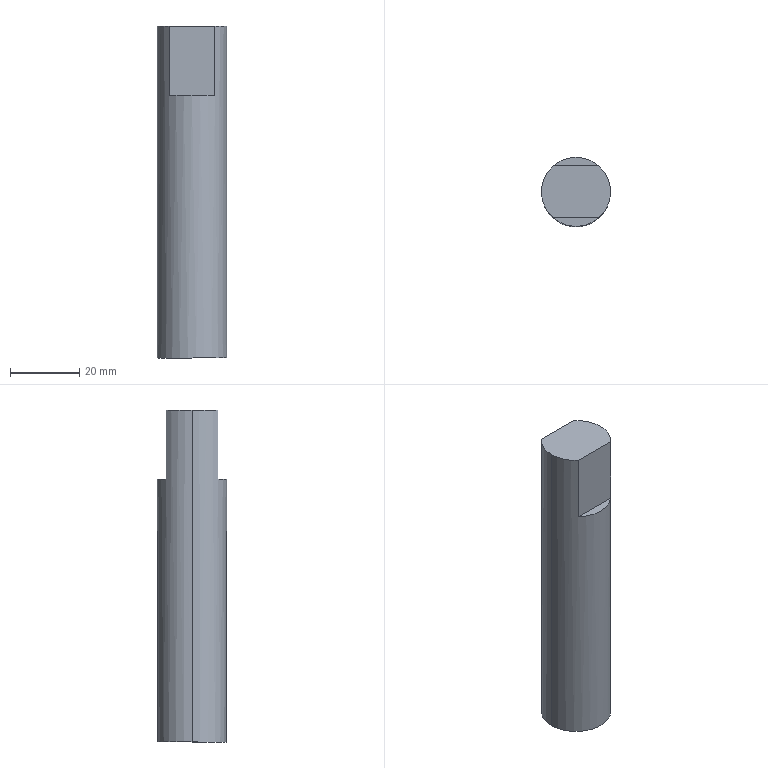Part | STEP file | 1 solid | 8 faces | box 20 x 20 x 96 mm | volume 29253 mm3 | plane 6 | cylinder 2 | commonest cylinder face diameters 20 x2
STEP:
#1=CARTESIAN_POINT('',(0.,0.,0.));
#2=DIRECTION('',(0.,0.,1.));
#3=DIRECTION('',(1.,0.,0.));
#4=AXIS2_PLACEMENT_3D('',#1,#2,#3);
#5=CARTESIAN_POINT('',(-51.732,1772.5,60.));
#6=VERTEX_POINT('',#5);
#7=CARTESIAN_POINT('',(-38.503,1772.5,60.));
#8=VERTEX_POINT('',#7);
#9=CARTESIAN_POINT('',(-45.117,1772.5,60.));
#10=DIRECTION('',(1.,0.,0.));
#11=VECTOR('',#10,1.);
#12=LINE('',#9,#11);
#13=CARTESIAN_POINT('',(-57.617,1772.5,40.));
#14=DIRECTION('',(0.,-1.,0.));
#15=DIRECTION('',(0.,0.,-1.));
#16=AXIS2_PLACEMENT_3D('',#13,#14,#15);
#17=PLANE('',#16);
#18=CARTESIAN_POINT('',(-20.,12.5));
#19=DIRECTION('',(0.,1.));
#20=VECTOR('',#19,1.);
#21=LINE('',#18,#20);
#22=(GEOMETRIC_REPRESENTATION_CONTEXT(2)PARAMETRIC_REPRESENTATION_CONTEXT()REPRESENTATION_CONTEXT('',''));
#23=DEFINITIONAL_REPRESENTATION('',(#21),#22);
#24=PCURVE('',#17,#23);
#25=CARTESIAN_POINT('',(-45.117,1780.,60.));
#26=DIRECTION('',(0.,0.,1.));
#27=DIRECTION('',(0.,-1.,0.));
#28=AXIS2_PLACEMENT_3D('',#25,#26,#27);
#29=PLANE('',#28);
#30=CARTESIAN_POINT('',(7.5,0.));
#31=DIRECTION('',(0.,1.));
#32=VECTOR('',#31,1.);
#33=LINE('',#30,#32);
#34=(GEOMETRIC_REPRESENTATION_CONTEXT(2)PARAMETRIC_REPRESENTATION_CONTEXT()REPRESENTATION_CONTEXT('',''));
#35=DEFINITIONAL_REPRESENTATION('',(#33),#34);
#36=PCURVE('',#29,#35);
#37=SURFACE_CURVE('',#12,(#24,#36),.PCURVE_S1.);
#38=EDGE_CURVE('',#6,#8,#37,.T.);
#39=ORIENTED_EDGE('',*,*,#38,.F.);
#40=CARTESIAN_POINT('',(-51.732,1772.5,40.));
#41=VERTEX_POINT('',#40);
#42=CARTESIAN_POINT('',(-51.732,1772.5,-36.));
#43=DIRECTION('',(0.,0.,1.));
#44=VECTOR('',#43,1.);
#45=LINE('',#42,#44);
#46=CARTESIAN_POINT('',(76.,5.886));
#47=DIRECTION('',(-1.,0.));
#48=VECTOR('',#47,1.);
#49=LINE('',#46,#48);
#50=(GEOMETRIC_REPRESENTATION_CONTEXT(2)PARAMETRIC_REPRESENTATION_CONTEXT()REPRESENTATION_CONTEXT('',''));
#51=DEFINITIONAL_REPRESENTATION('',(#49),#50);
#52=PCURVE('',#17,#51);
#53=CARTESIAN_POINT('',(-45.117,1780.,-36.));
#54=DIRECTION('',(0.,0.,1.));
#55=DIRECTION('',(1.,0.,0.));
#56=AXIS2_PLACEMENT_3D('',#53,#54,#55);
#57=CYLINDRICAL_SURFACE('',#56,10.);
#58=CARTESIAN_POINT('',(3.99,0.));
#59=DIRECTION('',(0.,1.));
#60=VECTOR('',#59,1.);
#61=LINE('',#58,#60);
#62=(GEOMETRIC_REPRESENTATION_CONTEXT(2)PARAMETRIC_REPRESENTATION_CONTEXT()REPRESENTATION_CONTEXT('',''));
#63=DEFINITIONAL_REPRESENTATION('',(#61),#62);
#64=PCURVE('',#57,#63);
#65=SURFACE_CURVE('',#45,(#52,#64),.PCURVE_S1.);
#66=EDGE_CURVE('',#41,#6,#65,.T.);
#67=ORIENTED_EDGE('',*,*,#66,.F.);
#68=CARTESIAN_POINT('',(-38.503,1772.5,40.));
#69=VERTEX_POINT('',#68);
#70=CARTESIAN_POINT('',(-57.617,1772.5,40.));
#71=DIRECTION('',(1.,0.,0.));
#72=VECTOR('',#71,1.);
#73=LINE('',#70,#72);
#74=CARTESIAN_POINT('',(0.,0.));
#75=DIRECTION('',(0.,1.));
#76=VECTOR('',#75,1.);
#77=LINE('',#74,#76);
#78=(GEOMETRIC_REPRESENTATION_CONTEXT(2)PARAMETRIC_REPRESENTATION_CONTEXT()REPRESENTATION_CONTEXT('',''));
#79=DEFINITIONAL_REPRESENTATION('',(#77),#78);
#80=PCURVE('',#17,#79);
#81=CARTESIAN_POINT('',(-45.117,1780.,40.));
#82=DIRECTION('',(0.,0.,1.));
#83=DIRECTION('',(1.,0.,0.));
#84=AXIS2_PLACEMENT_3D('',#81,#82,#83);
#85=PLANE('',#84);
#86=CARTESIAN_POINT('',(-12.5,-7.5));
#87=DIRECTION('',(1.,0.));
#88=VECTOR('',#87,1.);
#89=LINE('',#86,#88);
#90=(GEOMETRIC_REPRESENTATION_CONTEXT(2)PARAMETRIC_REPRESENTATION_CONTEXT()REPRESENTATION_CONTEXT('',''));
#91=DEFINITIONAL_REPRESENTATION('',(#89),#90);
#92=PCURVE('',#85,#91);
#93=SURFACE_CURVE('',#73,(#80,#92),.PCURVE_S1.);
#94=EDGE_CURVE('',#41,#69,#93,.T.);
#95=ORIENTED_EDGE('',*,*,#94,.T.);
#96=CARTESIAN_POINT('',(-38.503,1772.5,-36.));
#97=DIRECTION('',(0.,0.,-1.));
#98=VECTOR('',#97,1.);
#99=LINE('',#96,#98);
#100=CARTESIAN_POINT('',(76.,19.114));
#101=DIRECTION('',(1.,0.));
#102=VECTOR('',#101,1.);
#103=LINE('',#100,#102);
#104=(GEOMETRIC_REPRESENTATION_CONTEXT(2)PARAMETRIC_REPRESENTATION_CONTEXT()REPRESENTATION_CONTEXT('',''));
#105=DEFINITIONAL_REPRESENTATION('',(#103),#104);
#106=PCURVE('',#17,#105);
#107=CARTESIAN_POINT('',(5.435,0.));
#108=DIRECTION('',(0.,-1.));
#109=VECTOR('',#108,1.);
#110=LINE('',#107,#109);
#111=(GEOMETRIC_REPRESENTATION_CONTEXT(2)PARAMETRIC_REPRESENTATION_CONTEXT()REPRESENTATION_CONTEXT('',''));
#112=DEFINITIONAL_REPRESENTATION('',(#110),#111);
#113=PCURVE('',#57,#112);
#114=SURFACE_CURVE('',#99,(#106,#113),.PCURVE_S1.);
#115=EDGE_CURVE('',#8,#69,#114,.T.);
#116=ORIENTED_EDGE('',*,*,#115,.F.);
#117=EDGE_LOOP('',(#39,#67,#95,#116));
#118=FACE_BOUND('',#117,.T.);
#119=ADVANCED_FACE('',(#118),#17,.T.);
#120=ORIENTED_EDGE('',*,*,#94,.F.);
#121=CARTESIAN_POINT('',(-45.117,1780.,40.));
#122=DIRECTION('',(0.,0.,-1.));
#123=DIRECTION('',(1.,0.,0.));
#124=AXIS2_PLACEMENT_3D('',#121,#122,#123);
#125=CIRCLE('',#124,10.);
#126=CARTESIAN_POINT('',(10.,0.));
#127=CARTESIAN_POINT('',(10.,-17.321));
#128=CARTESIAN_POINT('',(-5.,-8.66));
#129=CARTESIAN_POINT('',(-20.,0.));
#130=CARTESIAN_POINT('',(-5.,8.66));
#131=CARTESIAN_POINT('',(10.,17.321));
#132=CARTESIAN_POINT('',(10.,0.));
#133=(BOUNDED_CURVE()B_SPLINE_CURVE(2,(#126,#127,#128,#129,#130,#131,#132),.UNSPECIFIED.,.T.,.F.)B_SPLINE_CURVE_WITH_KNOTS((1,2,2,2,2,1),(-2.094,0.,2.094,4.189,6.283,8.378),.UNSPECIFIED.)CURVE()GEOMETRIC_REPRESENTATION_ITEM()RATIONAL_B_SPLINE_CURVE((1.,0.5,1.,0.5,1.,0.5,1.))REPRESENTATION_ITEM(''));
#134=(GEOMETRIC_REPRESENTATION_CONTEXT(2)PARAMETRIC_REPRESENTATION_CONTEXT()REPRESENTATION_CONTEXT('',''));
#135=DEFINITIONAL_REPRESENTATION('',(#133),#134);
#136=PCURVE('',#85,#135);
#137=CARTESIAN_POINT('',(6.283,76.));
#138=DIRECTION('',(-1.,0.));
#139=VECTOR('',#138,1.);
#140=LINE('',#137,#139);
#141=(GEOMETRIC_REPRESENTATION_CONTEXT(2)PARAMETRIC_REPRESENTATION_CONTEXT()REPRESENTATION_CONTEXT('',''));
#142=DEFINITIONAL_REPRESENTATION('',(#140),#141);
#143=PCURVE('',#57,#142);
#144=SURFACE_CURVE('',#125,(#136,#143),.PCURVE_S1.);
#145=EDGE_CURVE('',#69,#41,#144,.T.);
#146=ORIENTED_EDGE('',*,*,#145,.F.);
#147=EDGE_LOOP('',(#120,#146));
#148=FACE_BOUND('',#147,.T.);
#149=ADVANCED_FACE('',(#148),#85,.T.);
#150=CARTESIAN_POINT('',(-38.503,1787.5,40.));
#151=VERTEX_POINT('',#150);
#152=CARTESIAN_POINT('',(-51.732,1787.5,40.));
#153=VERTEX_POINT('',#152);
#154=CARTESIAN_POINT('',(-57.617,1787.5,40.));
#155=DIRECTION('',(-1.,0.,0.));
#156=VECTOR('',#155,1.);
#157=LINE('',#154,#156);
#158=CARTESIAN_POINT('',(-45.117,1780.,40.));
#159=DIRECTION('',(0.,0.,1.));
#160=DIRECTION('',(1.,0.,0.));
#161=AXIS2_PLACEMENT_3D('',#158,#159,#160);
#162=PLANE('',#161);
#163=CARTESIAN_POINT('',(-12.5,7.5));
#164=DIRECTION('',(-1.,0.));
#165=VECTOR('',#164,1.);
#166=LINE('',#163,#165);
#167=(GEOMETRIC_REPRESENTATION_CONTEXT(2)PARAMETRIC_REPRESENTATION_CONTEXT()REPRESENTATION_CONTEXT('',''));
#168=DEFINITIONAL_REPRESENTATION('',(#166),#167);
#169=PCURVE('',#162,#168);
#170=CARTESIAN_POINT('',(-57.617,1787.5,40.));
#171=DIRECTION('',(0.,1.,0.));
#172=DIRECTION('',(1.,0.,0.));
#173=AXIS2_PLACEMENT_3D('',#170,#171,#172);
#174=PLANE('',#173);
#175=CARTESIAN_POINT('',(0.,0.));
#176=DIRECTION('',(-1.,0.));
#177=VECTOR('',#176,1.);
#178=LINE('',#175,#177);
#179=(GEOMETRIC_REPRESENTATION_CONTEXT(2)PARAMETRIC_REPRESENTATION_CONTEXT()REPRESENTATION_CONTEXT('',''));
#180=DEFINITIONAL_REPRESENTATION('',(#178),#179);
#181=PCURVE('',#174,#180);
#182=SURFACE_CURVE('',#157,(#169,#181),.PCURVE_S1.);
#183=EDGE_CURVE('',#151,#153,#182,.T.);
#184=ORIENTED_EDGE('',*,*,#183,.F.);
#185=CARTESIAN_POINT('',(-45.117,1780.,40.));
#186=DIRECTION('',(0.,0.,-1.));
#187=DIRECTION('',(1.,0.,0.));
#188=AXIS2_PLACEMENT_3D('',#185,#186,#187);
#189=CIRCLE('',#188,10.);
#190=CARTESIAN_POINT('',(10.,0.));
#191=CARTESIAN_POINT('',(10.,-17.321));
#192=CARTESIAN_POINT('',(-5.,-8.66));
#193=CARTESIAN_POINT('',(-20.,0.));
#194=CARTESIAN_POINT('',(-5.,8.66));
#195=CARTESIAN_POINT('',(10.,17.321));
#196=CARTESIAN_POINT('',(10.,0.));
#197=(BOUNDED_CURVE()B_SPLINE_CURVE(2,(#190,#191,#192,#193,#194,#195,#196),.UNSPECIFIED.,.T.,.F.)B_SPLINE_CURVE_WITH_KNOTS((1,2,2,2,2,1),(-2.094,0.,2.094,4.189,6.283,8.378),.UNSPECIFIED.)CURVE()GEOMETRIC_REPRESENTATION_ITEM()RATIONAL_B_SPLINE_CURVE((1.,0.5,1.,0.5,1.,0.5,1.))REPRESENTATION_ITEM(''));
#198=(GEOMETRIC_REPRESENTATION_CONTEXT(2)PARAMETRIC_REPRESENTATION_CONTEXT()REPRESENTATION_CONTEXT('',''));
#199=DEFINITIONAL_REPRESENTATION('',(#197),#198);
#200=PCURVE('',#162,#199);
#201=CARTESIAN_POINT('',(-45.117,1780.,-36.));
#202=DIRECTION('',(0.,0.,1.));
#203=DIRECTION('',(1.,0.,0.));
#204=AXIS2_PLACEMENT_3D('',#201,#202,#203);
#205=CYLINDRICAL_SURFACE('',#204,10.);
#206=CARTESIAN_POINT('',(6.283,76.));
#207=DIRECTION('',(-1.,0.));
#208=VECTOR('',#207,1.);
#209=LINE('',#206,#208);
#210=(GEOMETRIC_REPRESENTATION_CONTEXT(2)PARAMETRIC_REPRESENTATION_CONTEXT()REPRESENTATION_CONTEXT('',''));
#211=DEFINITIONAL_REPRESENTATION('',(#209),#210);
#212=PCURVE('',#205,#211);
#213=SURFACE_CURVE('',#189,(#200,#212),.PCURVE_S1.);
#214=EDGE_CURVE('',#153,#151,#213,.T.);
#215=ORIENTED_EDGE('',*,*,#214,.F.);
#216=EDGE_LOOP('',(#184,#215));
#217=FACE_BOUND('',#216,.T.);
#218=ADVANCED_FACE('',(#217),#162,.T.);
#219=CARTESIAN_POINT('',(-38.503,1787.5,60.));
#220=VERTEX_POINT('',#219);
#221=CARTESIAN_POINT('',(-51.732,1787.5,60.));
#222=VERTEX_POINT('',#221);
#223=CARTESIAN_POINT('',(-45.117,1787.5,60.));
#224=DIRECTION('',(-1.,0.,0.));
#225=VECTOR('',#224,1.);
#226=LINE('',#223,#225);
#227=CARTESIAN_POINT('',(12.5,-20.));
#228=DIRECTION('',(-1.,0.));
#229=VECTOR('',#228,1.);
#230=LINE('',#227,#229);
#231=(GEOMETRIC_REPRESENTATION_CONTEXT(2)PARAMETRIC_REPRESENTATION_CONTEXT()REPRESENTATION_CONTEXT('',''));
#232=DEFINITIONAL_REPRESENTATION('',(#230),#231);
#233=PCURVE('',#174,#232);
#234=CARTESIAN_POINT('',(-7.5,0.));
#235=DIRECTION('',(0.,-1.));
#236=VECTOR('',#235,1.);
#237=LINE('',#234,#236);
#238=(GEOMETRIC_REPRESENTATION_CONTEXT(2)PARAMETRIC_REPRESENTATION_CONTEXT()REPRESENTATION_CONTEXT('',''));
#239=DEFINITIONAL_REPRESENTATION('',(#237),#238);
#240=PCURVE('',#29,#239);
#241=SURFACE_CURVE('',#226,(#233,#240),.PCURVE_S1.);
#242=EDGE_CURVE('',#220,#222,#241,.T.);
#243=ORIENTED_EDGE('',*,*,#242,.F.);
#244=CARTESIAN_POINT('',(-38.503,1787.5,-36.));
#245=DIRECTION('',(0.,0.,1.));
#246=VECTOR('',#245,1.);
#247=LINE('',#244,#246);
#248=CARTESIAN_POINT('',(19.114,76.));
#249=DIRECTION('',(0.,-1.));
#250=VECTOR('',#249,1.);
#251=LINE('',#248,#250);
#252=(GEOMETRIC_REPRESENTATION_CONTEXT(2)PARAMETRIC_REPRESENTATION_CONTEXT()REPRESENTATION_CONTEXT('',''));
#253=DEFINITIONAL_REPRESENTATION('',(#251),#252);
#254=PCURVE('',#174,#253);
#255=CARTESIAN_POINT('',(0.8481,0.));
#256=DIRECTION('',(0.,1.));
#257=VECTOR('',#256,1.);
#258=LINE('',#255,#257);
#259=(GEOMETRIC_REPRESENTATION_CONTEXT(2)PARAMETRIC_REPRESENTATION_CONTEXT()REPRESENTATION_CONTEXT('',''));
#260=DEFINITIONAL_REPRESENTATION('',(#258),#259);
#261=PCURVE('',#205,#260);
#262=SURFACE_CURVE('',#247,(#254,#261),.PCURVE_S1.);
#263=EDGE_CURVE('',#151,#220,#262,.T.);
#264=ORIENTED_EDGE('',*,*,#263,.F.);
#265=ORIENTED_EDGE('',*,*,#183,.T.);
#266=CARTESIAN_POINT('',(-51.732,1787.5,-36.));
#267=DIRECTION('',(0.,0.,-1.));
#268=VECTOR('',#267,1.);
#269=LINE('',#266,#268);
#270=CARTESIAN_POINT('',(5.886,76.));
#271=DIRECTION('',(0.,1.));
#272=VECTOR('',#271,1.);
#273=LINE('',#270,#272);
#274=(GEOMETRIC_REPRESENTATION_CONTEXT(2)PARAMETRIC_REPRESENTATION_CONTEXT()REPRESENTATION_CONTEXT('',''));
#275=DEFINITIONAL_REPRESENTATION('',(#273),#274);
#276=PCURVE('',#174,#275);
#277=CARTESIAN_POINT('',(2.294,0.));
#278=DIRECTION('',(0.,-1.));
#279=VECTOR('',#278,1.);
#280=LINE('',#277,#279);
#281=(GEOMETRIC_REPRESENTATION_CONTEXT(2)PARAMETRIC_REPRESENTATION_CONTEXT()REPRESENTATION_CONTEXT('',''));
#282=DEFINITIONAL_REPRESENTATION('',(#280),#281);
#283=PCURVE('',#205,#282);
#284=SURFACE_CURVE('',#269,(#276,#283),.PCURVE_S1.);
#285=EDGE_CURVE('',#222,#153,#284,.T.);
#286=ORIENTED_EDGE('',*,*,#285,.F.);
#287=EDGE_LOOP('',(#243,#264,#265,#286));
#288=FACE_BOUND('',#287,.T.);
#289=ADVANCED_FACE('',(#288),#174,.T.);
#290=CARTESIAN_POINT('',(-35.117,1780.,-36.));
#291=VERTEX_POINT('',#290);
#292=CARTESIAN_POINT('',(-55.117,1780.,-36.));
#293=VERTEX_POINT('',#292);
#294=CARTESIAN_POINT('',(-45.117,1780.,-36.));
#295=DIRECTION('',(0.,0.,1.));
#296=DIRECTION('',(1.,0.,0.));
#297=AXIS2_PLACEMENT_3D('',#294,#295,#296);
#298=CIRCLE('',#297,10.);
#299=CARTESIAN_POINT('',(-45.117,1780.,-36.));
#300=DIRECTION('',(0.,0.,1.));
#301=DIRECTION('',(0.,-1.,0.));
#302=AXIS2_PLACEMENT_3D('',#299,#300,#301);
#303=PLANE('',#302);
#304=CARTESIAN_POINT('',(0.,0.));
#305=DIRECTION('',(0.,1.));
#306=AXIS2_PLACEMENT_2D('',#304,#305);
#307=CIRCLE('',#306,10.);
#308=(GEOMETRIC_REPRESENTATION_CONTEXT(2)PARAMETRIC_REPRESENTATION_CONTEXT()REPRESENTATION_CONTEXT('',''));
#309=DEFINITIONAL_REPRESENTATION('',(#307),#308);
#310=PCURVE('',#303,#309);
#311=CARTESIAN_POINT('',(0.,0.));
#312=DIRECTION('',(1.,0.));
#313=VECTOR('',#312,1.);
#314=LINE('',#311,#313);
#315=(GEOMETRIC_REPRESENTATION_CONTEXT(2)PARAMETRIC_REPRESENTATION_CONTEXT()REPRESENTATION_CONTEXT('',''));
#316=DEFINITIONAL_REPRESENTATION('',(#314),#315);
#317=PCURVE('',#205,#316);
#318=SURFACE_CURVE('',#298,(#310,#317),.PCURVE_S1.);
#319=EDGE_CURVE('',#291,#293,#318,.T.);
#320=ORIENTED_EDGE('',*,*,#319,.F.);
#321=CARTESIAN_POINT('',(-45.117,1780.,-36.));
#322=DIRECTION('',(0.,0.,1.));
#323=DIRECTION('',(1.,0.,0.));
#324=AXIS2_PLACEMENT_3D('',#321,#322,#323);
#325=CIRCLE('',#324,10.);
#326=CARTESIAN_POINT('',(0.,0.));
#327=DIRECTION('',(0.,1.));
#328=AXIS2_PLACEMENT_2D('',#326,#327);
#329=CIRCLE('',#328,10.);
#330=(GEOMETRIC_REPRESENTATION_CONTEXT(2)PARAMETRIC_REPRESENTATION_CONTEXT()REPRESENTATION_CONTEXT('',''));
#331=DEFINITIONAL_REPRESENTATION('',(#329),#330);
#332=PCURVE('',#303,#331);
#333=CARTESIAN_POINT('',(0.,0.));
#334=DIRECTION('',(1.,0.));
#335=VECTOR('',#334,1.);
#336=LINE('',#333,#335);
#337=(GEOMETRIC_REPRESENTATION_CONTEXT(2)PARAMETRIC_REPRESENTATION_CONTEXT()REPRESENTATION_CONTEXT('',''));
#338=DEFINITIONAL_REPRESENTATION('',(#336),#337);
#339=PCURVE('',#57,#338);
#340=SURFACE_CURVE('',#325,(#332,#339),.PCURVE_S1.);
#341=EDGE_CURVE('',#293,#291,#340,.T.);
#342=ORIENTED_EDGE('',*,*,#341,.F.);
#343=EDGE_LOOP('',(#320,#342));
#344=FACE_BOUND('',#343,.T.);
#345=ADVANCED_FACE('',(#344),#303,.F.);
#346=CARTESIAN_POINT('',(-55.117,1780.,60.));
#347=VERTEX_POINT('',#346);
#348=CARTESIAN_POINT('',(-45.117,1780.,60.));
#349=DIRECTION('',(0.,0.,1.));
#350=DIRECTION('',(1.,0.,0.));
#351=AXIS2_PLACEMENT_3D('',#348,#349,#350);
#352=CIRCLE('',#351,10.);
#353=CARTESIAN_POINT('',(0.,0.));
#354=DIRECTION('',(0.,1.));
#355=AXIS2_PLACEMENT_2D('',#353,#354);
#356=CIRCLE('',#355,10.);
#357=(GEOMETRIC_REPRESENTATION_CONTEXT(2)PARAMETRIC_REPRESENTATION_CONTEXT()REPRESENTATION_CONTEXT('',''));
#358=DEFINITIONAL_REPRESENTATION('',(#356),#357);
#359=PCURVE('',#29,#358);
#360=CARTESIAN_POINT('',(0.,96.));
#361=DIRECTION('',(1.,0.));
#362=VECTOR('',#361,1.);
#363=LINE('',#360,#362);
#364=(GEOMETRIC_REPRESENTATION_CONTEXT(2)PARAMETRIC_REPRESENTATION_CONTEXT()REPRESENTATION_CONTEXT('',''));
#365=DEFINITIONAL_REPRESENTATION('',(#363),#364);
#366=PCURVE('',#205,#365);
#367=SURFACE_CURVE('',#352,(#359,#366),.PCURVE_S1.);
#368=EDGE_CURVE('',#222,#347,#367,.T.);
#369=ORIENTED_EDGE('',*,*,#368,.T.);
#370=CARTESIAN_POINT('',(-45.117,1780.,60.));
#371=DIRECTION('',(0.,0.,1.));
#372=DIRECTION('',(1.,0.,0.));
#373=AXIS2_PLACEMENT_3D('',#370,#371,#372);
#374=CIRCLE('',#373,10.);
#375=CARTESIAN_POINT('',(0.,0.));
#376=DIRECTION('',(0.,1.));
#377=AXIS2_PLACEMENT_2D('',#375,#376);
#378=CIRCLE('',#377,10.);
#379=(GEOMETRIC_REPRESENTATION_CONTEXT(2)PARAMETRIC_REPRESENTATION_CONTEXT()REPRESENTATION_CONTEXT('',''));
#380=DEFINITIONAL_REPRESENTATION('',(#378),#379);
#381=PCURVE('',#29,#380);
#382=CARTESIAN_POINT('',(0.,96.));
#383=DIRECTION('',(1.,0.));
#384=VECTOR('',#383,1.);
#385=LINE('',#382,#384);
#386=(GEOMETRIC_REPRESENTATION_CONTEXT(2)PARAMETRIC_REPRESENTATION_CONTEXT()REPRESENTATION_CONTEXT('',''));
#387=DEFINITIONAL_REPRESENTATION('',(#385),#386);
#388=PCURVE('',#57,#387);
#389=SURFACE_CURVE('',#374,(#381,#388),.PCURVE_S1.);
#390=EDGE_CURVE('',#347,#6,#389,.T.);
#391=ORIENTED_EDGE('',*,*,#390,.T.);
#392=ORIENTED_EDGE('',*,*,#38,.T.);
#393=CARTESIAN_POINT('',(-35.117,1780.,60.));
#394=VERTEX_POINT('',#393);
#395=CARTESIAN_POINT('',(-45.117,1780.,60.));
#396=DIRECTION('',(0.,0.,1.));
#397=DIRECTION('',(1.,0.,0.));
#398=AXIS2_PLACEMENT_3D('',#395,#396,#397);
#399=CIRCLE('',#398,10.);
#400=CARTESIAN_POINT('',(0.,0.));
#401=DIRECTION('',(0.,1.));
#402=AXIS2_PLACEMENT_2D('',#400,#401);
#403=CIRCLE('',#402,10.);
#404=(GEOMETRIC_REPRESENTATION_CONTEXT(2)PARAMETRIC_REPRESENTATION_CONTEXT()REPRESENTATION_CONTEXT('',''));
#405=DEFINITIONAL_REPRESENTATION('',(#403),#404);
#406=PCURVE('',#29,#405);
#407=CARTESIAN_POINT('',(0.,96.));
#408=DIRECTION('',(1.,0.));
#409=VECTOR('',#408,1.);
#410=LINE('',#407,#409);
#411=(GEOMETRIC_REPRESENTATION_CONTEXT(2)PARAMETRIC_REPRESENTATION_CONTEXT()REPRESENTATION_CONTEXT('',''));
#412=DEFINITIONAL_REPRESENTATION('',(#410),#411);
#413=PCURVE('',#57,#412);
#414=SURFACE_CURVE('',#399,(#406,#413),.PCURVE_S1.);
#415=EDGE_CURVE('',#8,#394,#414,.T.);
#416=ORIENTED_EDGE('',*,*,#415,.T.);
#417=CARTESIAN_POINT('',(-45.117,1780.,60.));
#418=DIRECTION('',(0.,0.,1.));
#419=DIRECTION('',(1.,0.,0.));
#420=AXIS2_PLACEMENT_3D('',#417,#418,#419);
#421=CIRCLE('',#420,10.);
#422=CARTESIAN_POINT('',(0.,0.));
#423=DIRECTION('',(0.,1.));
#424=AXIS2_PLACEMENT_2D('',#422,#423);
#425=CIRCLE('',#424,10.);
#426=(GEOMETRIC_REPRESENTATION_CONTEXT(2)PARAMETRIC_REPRESENTATION_CONTEXT()REPRESENTATION_CONTEXT('',''));
#427=DEFINITIONAL_REPRESENTATION('',(#425),#426);
#428=PCURVE('',#29,#427);
#429=CARTESIAN_POINT('',(0.,96.));
#430=DIRECTION('',(1.,0.));
#431=VECTOR('',#430,1.);
#432=LINE('',#429,#431);
#433=(GEOMETRIC_REPRESENTATION_CONTEXT(2)PARAMETRIC_REPRESENTATION_CONTEXT()REPRESENTATION_CONTEXT('',''));
#434=DEFINITIONAL_REPRESENTATION('',(#432),#433);
#435=PCURVE('',#205,#434);
#436=SURFACE_CURVE('',#421,(#428,#435),.PCURVE_S1.);
#437=EDGE_CURVE('',#394,#220,#436,.T.);
#438=ORIENTED_EDGE('',*,*,#437,.T.);
#439=ORIENTED_EDGE('',*,*,#242,.T.);
#440=EDGE_LOOP('',(#369,#391,#392,#416,#438,#439));
#441=FACE_BOUND('',#440,.T.);
#442=ADVANCED_FACE('',(#441),#29,.T.);
#443=CARTESIAN_POINT('',(-55.117,1780.,-36.));
#444=DIRECTION('',(0.,0.,1.));
#445=VECTOR('',#444,1.);
#446=LINE('',#443,#445);
#447=CARTESIAN_POINT('',(3.142,0.));
#448=DIRECTION('',(0.,1.));
#449=VECTOR('',#448,1.);
#450=LINE('',#447,#449);
#451=(GEOMETRIC_REPRESENTATION_CONTEXT(2)PARAMETRIC_REPRESENTATION_CONTEXT()REPRESENTATION_CONTEXT('',''));
#452=DEFINITIONAL_REPRESENTATION('',(#450),#451);
#453=PCURVE('',#57,#452);
#454=CARTESIAN_POINT('',(3.142,0.));
#455=DIRECTION('',(0.,1.));
#456=VECTOR('',#455,1.);
#457=LINE('',#454,#456);
#458=(GEOMETRIC_REPRESENTATION_CONTEXT(2)PARAMETRIC_REPRESENTATION_CONTEXT()REPRESENTATION_CONTEXT('',''));
#459=DEFINITIONAL_REPRESENTATION('',(#457),#458);
#460=PCURVE('',#205,#459);
#461=SURFACE_CURVE('',#446,(#453,#460),.PCURVE_S1.);
#462=EDGE_CURVE('',#293,#347,#461,.T.);
#463=ORIENTED_EDGE('',*,*,#462,.F.);
#464=ORIENTED_EDGE('',*,*,#341,.T.);
#465=CARTESIAN_POINT('',(-35.117,1780.,-36.));
#466=DIRECTION('',(0.,0.,1.));
#467=VECTOR('',#466,1.);
#468=LINE('',#465,#467);
#469=CARTESIAN_POINT('',(6.283,0.));
#470=DIRECTION('',(0.,1.));
#471=VECTOR('',#470,1.);
#472=LINE('',#469,#471);
#473=(GEOMETRIC_REPRESENTATION_CONTEXT(2)PARAMETRIC_REPRESENTATION_CONTEXT()REPRESENTATION_CONTEXT('',''));
#474=DEFINITIONAL_REPRESENTATION('',(#472),#473);
#475=PCURVE('',#57,#474);
#476=CARTESIAN_POINT('',(0.,0.));
#477=DIRECTION('',(0.,1.));
#478=VECTOR('',#477,1.);
#479=LINE('',#476,#478);
#480=(GEOMETRIC_REPRESENTATION_CONTEXT(2)PARAMETRIC_REPRESENTATION_CONTEXT()REPRESENTATION_CONTEXT('',''));
#481=DEFINITIONAL_REPRESENTATION('',(#479),#480);
#482=PCURVE('',#205,#481);
#483=SURFACE_CURVE('',#468,(#475,#482),.PCURVE_S1.);
#484=EDGE_CURVE('',#291,#394,#483,.T.);
#485=ORIENTED_EDGE('',*,*,#484,.T.);
#486=ORIENTED_EDGE('',*,*,#415,.F.);
#487=ORIENTED_EDGE('',*,*,#115,.T.);
#488=ORIENTED_EDGE('',*,*,#145,.T.);
#489=ORIENTED_EDGE('',*,*,#66,.T.);
#490=ORIENTED_EDGE('',*,*,#390,.F.);
#491=EDGE_LOOP('',(#463,#464,#485,#486,#487,#488,#489,#490));
#492=FACE_BOUND('',#491,.T.);
#493=ADVANCED_FACE('',(#492),#57,.T.);
#494=ORIENTED_EDGE('',*,*,#319,.T.);
#495=ORIENTED_EDGE('',*,*,#462,.T.);
#496=ORIENTED_EDGE('',*,*,#368,.F.);
#497=ORIENTED_EDGE('',*,*,#285,.T.);
#498=ORIENTED_EDGE('',*,*,#214,.T.);
#499=ORIENTED_EDGE('',*,*,#263,.T.);
#500=ORIENTED_EDGE('',*,*,#437,.F.);
#501=ORIENTED_EDGE('',*,*,#484,.F.);
#502=EDGE_LOOP('',(#494,#495,#496,#497,#498,#499,#500,#501));
#503=FACE_BOUND('',#502,.T.);
#504=ADVANCED_FACE('',(#503),#205,.T.);
#505=CLOSED_SHELL('',(#119,#149,#218,#289,#345,#442,#493,#504));
#506=MANIFOLD_SOLID_BREP('',#505);
#507=(LENGTH_UNIT()NAMED_UNIT(*)SI_UNIT(.MILLI.,.METRE.));
#508=UNCERTAINTY_MEASURE_WITH_UNIT(LENGTH_MEASURE(0.0000001),#507,'','');
#509=(NAMED_UNIT(*)PLANE_ANGLE_UNIT()SI_UNIT($,.RADIAN.));
#510=(NAMED_UNIT(*)SI_UNIT($,.STERADIAN.)SOLID_ANGLE_UNIT());
#511=(GEOMETRIC_REPRESENTATION_CONTEXT(3)GLOBAL_UNCERTAINTY_ASSIGNED_CONTEXT((#508))GLOBAL_UNIT_ASSIGNED_CONTEXT((#507,#509,#510))REPRESENTATION_CONTEXT('',''));
#512=ADVANCED_BREP_SHAPE_REPRESENTATION('',(#4,#506),#511);